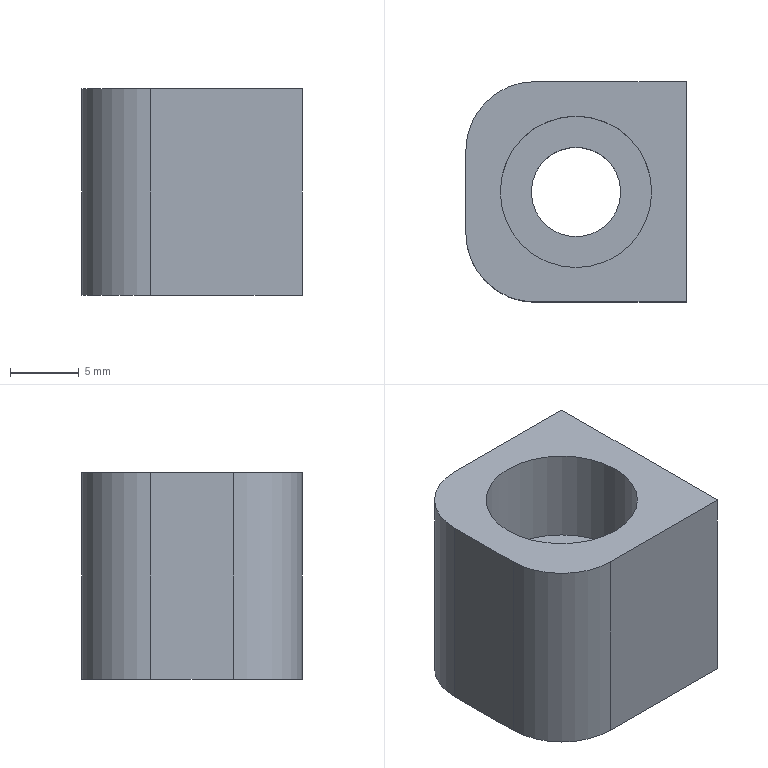Part | STEP file | solid 42 | 1 solid | 11 faces | box 16 x 16 x 15 mm | volume 2748 mm3 | plane 7 | cylinder 4 | commonest cylinder face diameters 10 x2 6.5 x1 11 x1